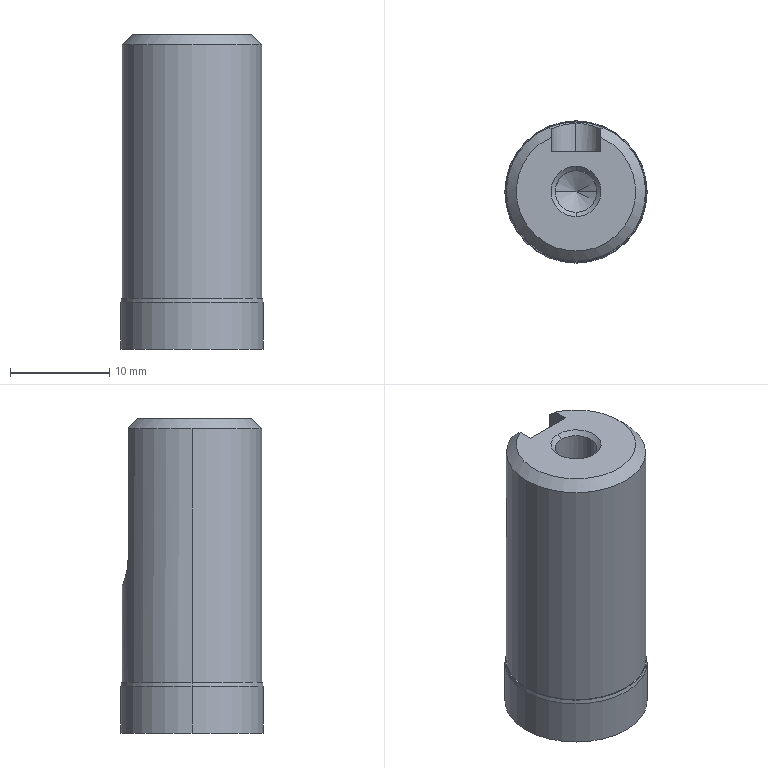Part | STEP file | _60-1-SO0001_1_1_1 | 1 solid | 24 faces | box 14.3 x 14.3 x 31.6 mm | volume 4477 mm3 | cylinder 8 | plane 8 | cone 7 | spline 1 | commonest cylinder face diameters 4.2 x2 5 x2 14 x2 14.3 x2